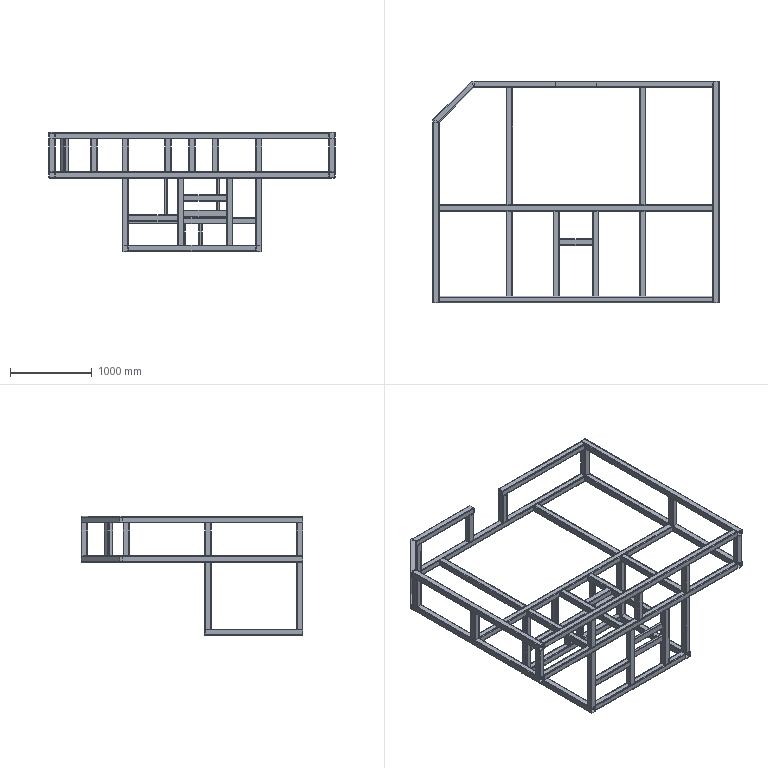Part | SolidWorks | features WeldCornerFeat 9, WeldMemberFeat 5, MoveCopyBody 4, ICE 2, 3DProfileFeature 1, EndCap 1, HoleWzd 1, WeldmentFeature 1 | 60 solids | 1008 faces | box 3500 x 2710 x 1460 mm | volume 76195969 mm3 | plane 572 | cylinder 436 | commonest cylinder face diameters 10 x193 20 x193 6 x16 12 x16 8 x8 16 x8